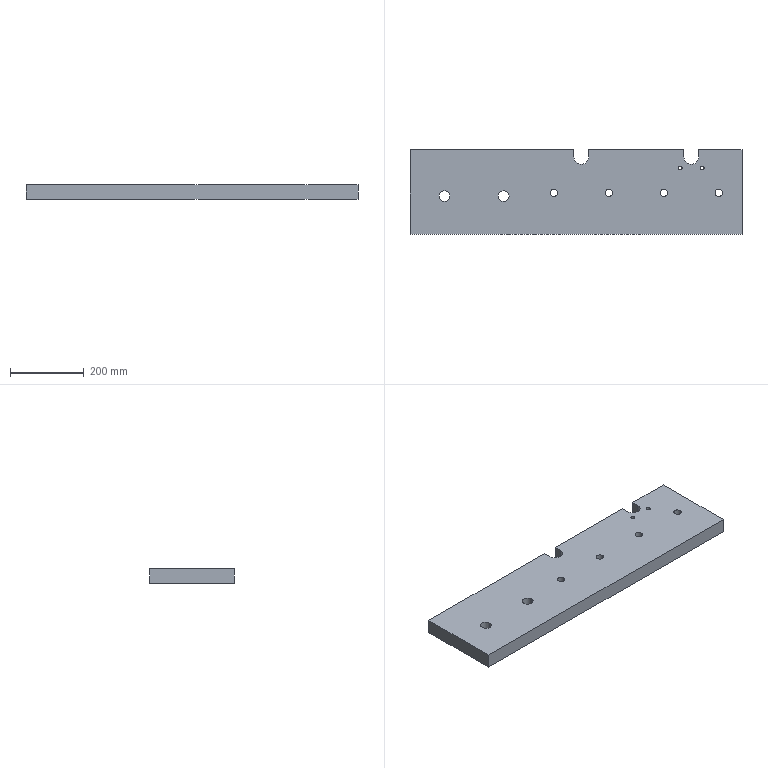Part | SolidWorks | features ICE 4, LPattern 2, Extrusion 1 | 1 solid | 30 faces | box 900 x 230 x 40 mm | volume 8056344 mm3 | cylinder 18 | plane 12 | commonest cylinder face diameters 20 x8 10 x4 29 x4 40 x2
STEP:
#1=CARTESIAN_POINT('',(-341.6,-11.,20.));
#2=VERTEX_POINT('',#1);
#3=CARTESIAN_POINT('',(-370.6,-11.,20.));
#4=VERTEX_POINT('',#3);
#5=CARTESIAN_POINT('',(-356.1,-11.,20.));
#6=DIRECTION('',(0.,0.,-1.));
#7=DIRECTION('',(-1.,0.,0.));
#8=AXIS2_PLACEMENT_3D('',#5,#6,#7);
#9=CIRCLE('',#8,14.5);
#10=EDGE_CURVE('',#2,#4,#9,.T.);
#11=ORIENTED_EDGE('',*,*,#10,.F.);
#12=CARTESIAN_POINT('',(-341.6,-11.,-20.));
#13=VERTEX_POINT('',#12);
#14=CARTESIAN_POINT('',(-341.6,-11.,20.));
#15=DIRECTION('',(0.,0.,-1.));
#16=VECTOR('',#15,1000.);
#17=LINE('',#14,#16);
#18=EDGE_CURVE('',#2,#13,#17,.T.);
#19=ORIENTED_EDGE('',*,*,#18,.T.);
#20=CARTESIAN_POINT('',(-370.6,-11.,-20.));
#21=VERTEX_POINT('',#20);
#22=CARTESIAN_POINT('',(-356.1,-11.,-20.));
#23=DIRECTION('',(0.,0.,-1.));
#24=DIRECTION('',(-1.,0.,0.));
#25=AXIS2_PLACEMENT_3D('',#22,#23,#24);
#26=CIRCLE('',#25,14.5);
#27=EDGE_CURVE('',#13,#21,#26,.T.);
#28=ORIENTED_EDGE('',*,*,#27,.T.);
#29=CARTESIAN_POINT('',(-370.6,-11.,20.));
#30=DIRECTION('',(0.,0.,-1.));
#31=VECTOR('',#30,1000.);
#32=LINE('',#29,#31);
#33=EDGE_CURVE('',#4,#21,#32,.T.);
#34=ORIENTED_EDGE('',*,*,#33,.F.);
#35=EDGE_LOOP('',(#11,#19,#28,#34));
#36=FACE_OUTER_BOUND('',#35,.T.);
#37=CARTESIAN_POINT('',(-356.1,-11.,20.));
#38=DIRECTION('',(0.,0.,-1.));
#39=DIRECTION('',(-1.,0.,0.));
#40=AXIS2_PLACEMENT_3D('',#37,#38,#39);
#41=CYLINDRICAL_SURFACE('',#40,14.5);
#42=ADVANCED_FACE('',(#36),#41,.F.);
#43=CARTESIAN_POINT('',(-181.6,-11.,20.));
#44=VERTEX_POINT('',#43);
#45=CARTESIAN_POINT('',(-210.6,-11.,20.));
#46=VERTEX_POINT('',#45);
#47=CARTESIAN_POINT('',(-196.1,-11.,20.));
#48=DIRECTION('',(0.,0.,-1.));
#49=DIRECTION('',(-1.,0.,0.));
#50=AXIS2_PLACEMENT_3D('',#47,#48,#49);
#51=CIRCLE('',#50,14.5);
#52=EDGE_CURVE('',#44,#46,#51,.T.);
#53=ORIENTED_EDGE('',*,*,#52,.F.);
#54=CARTESIAN_POINT('',(-181.6,-11.,-20.));
#55=VERTEX_POINT('',#54);
#56=CARTESIAN_POINT('',(-181.6,-11.,20.));
#57=DIRECTION('',(0.,0.,-1.));
#58=VECTOR('',#57,1000.);
#59=LINE('',#56,#58);
#60=EDGE_CURVE('',#44,#55,#59,.T.);
#61=ORIENTED_EDGE('',*,*,#60,.T.);
#62=CARTESIAN_POINT('',(-210.6,-11.,-20.));
#63=VERTEX_POINT('',#62);
#64=CARTESIAN_POINT('',(-196.1,-11.,-20.));
#65=DIRECTION('',(0.,0.,-1.));
#66=DIRECTION('',(-1.,0.,0.));
#67=AXIS2_PLACEMENT_3D('',#64,#65,#66);
#68=CIRCLE('',#67,14.5);
#69=EDGE_CURVE('',#55,#63,#68,.T.);
#70=ORIENTED_EDGE('',*,*,#69,.T.);
#71=CARTESIAN_POINT('',(-210.6,-11.,20.));
#72=DIRECTION('',(0.,0.,-1.));
#73=VECTOR('',#72,1000.);
#74=LINE('',#71,#73);
#75=EDGE_CURVE('',#46,#63,#74,.T.);
#76=ORIENTED_EDGE('',*,*,#75,.F.);
#77=EDGE_LOOP('',(#53,#61,#70,#76));
#78=FACE_OUTER_BOUND('',#77,.T.);
#79=CARTESIAN_POINT('',(-196.1,-11.,20.));
#80=DIRECTION('',(0.,0.,-1.));
#81=DIRECTION('',(-1.,0.,0.));
#82=AXIS2_PLACEMENT_3D('',#79,#80,#81);
#83=CYLINDRICAL_SURFACE('',#82,14.5);
#84=ADVANCED_FACE('',(#78),#83,.F.);
#85=CARTESIAN_POINT('',(347.5,65.,20.));
#86=VERTEX_POINT('',#85);
#87=CARTESIAN_POINT('',(337.5,65.,20.));
#88=VERTEX_POINT('',#87);
#89=CARTESIAN_POINT('',(342.5,65.,20.));
#90=DIRECTION('',(0.,0.,-1.));
#91=DIRECTION('',(-1.,0.,0.));
#92=AXIS2_PLACEMENT_3D('',#89,#90,#91);
#93=CIRCLE('',#92,5.);
#94=EDGE_CURVE('',#86,#88,#93,.T.);
#95=ORIENTED_EDGE('',*,*,#94,.F.);
#96=CARTESIAN_POINT('',(347.5,65.,-20.));
#97=VERTEX_POINT('',#96);
#98=CARTESIAN_POINT('',(347.5,65.,20.));
#99=DIRECTION('',(0.,0.,-1.));
#100=VECTOR('',#99,1000.);
#101=LINE('',#98,#100);
#102=EDGE_CURVE('',#86,#97,#101,.T.);
#103=ORIENTED_EDGE('',*,*,#102,.T.);
#104=CARTESIAN_POINT('',(337.5,65.,-20.));
#105=VERTEX_POINT('',#104);
#106=CARTESIAN_POINT('',(342.5,65.,-20.));
#107=DIRECTION('',(0.,0.,-1.));
#108=DIRECTION('',(-1.,0.,0.));
#109=AXIS2_PLACEMENT_3D('',#106,#107,#108);
#110=CIRCLE('',#109,5.);
#111=EDGE_CURVE('',#97,#105,#110,.T.);
#112=ORIENTED_EDGE('',*,*,#111,.T.);
#113=CARTESIAN_POINT('',(337.5,65.,20.));
#114=DIRECTION('',(0.,0.,-1.));
#115=VECTOR('',#114,1000.);
#116=LINE('',#113,#115);
#117=EDGE_CURVE('',#88,#105,#116,.T.);
#118=ORIENTED_EDGE('',*,*,#117,.F.);
#119=EDGE_LOOP('',(#95,#103,#112,#118));
#120=FACE_OUTER_BOUND('',#119,.T.);
#121=CARTESIAN_POINT('',(342.5,65.,20.));
#122=DIRECTION('',(0.,0.,-1.));
#123=DIRECTION('',(-1.,0.,0.));
#124=AXIS2_PLACEMENT_3D('',#121,#122,#123);
#125=CYLINDRICAL_SURFACE('',#124,5.);
#126=ADVANCED_FACE('',(#120),#125,.F.);
#127=CARTESIAN_POINT('',(287.5,65.,20.));
#128=VERTEX_POINT('',#127);
#129=CARTESIAN_POINT('',(277.5,65.,20.));
#130=VERTEX_POINT('',#129);
#131=CARTESIAN_POINT('',(282.5,65.,20.));
#132=DIRECTION('',(0.,0.,-1.));
#133=DIRECTION('',(1.,0.,0.));
#134=AXIS2_PLACEMENT_3D('',#131,#132,#133);
#135=CIRCLE('',#134,5.);
#136=EDGE_CURVE('',#128,#130,#135,.T.);
#137=ORIENTED_EDGE('',*,*,#136,.F.);
#138=CARTESIAN_POINT('',(287.5,65.,-20.));
#139=VERTEX_POINT('',#138);
#140=CARTESIAN_POINT('',(287.5,65.,20.));
#141=DIRECTION('',(0.,0.,-1.));
#142=VECTOR('',#141,1000.);
#143=LINE('',#140,#142);
#144=EDGE_CURVE('',#128,#139,#143,.T.);
#145=ORIENTED_EDGE('',*,*,#144,.T.);
#146=CARTESIAN_POINT('',(277.5,65.,-20.));
#147=VERTEX_POINT('',#146);
#148=CARTESIAN_POINT('',(282.5,65.,-20.));
#149=DIRECTION('',(0.,0.,-1.));
#150=DIRECTION('',(1.,0.,0.));
#151=AXIS2_PLACEMENT_3D('',#148,#149,#150);
#152=CIRCLE('',#151,5.);
#153=EDGE_CURVE('',#139,#147,#152,.T.);
#154=ORIENTED_EDGE('',*,*,#153,.T.);
#155=CARTESIAN_POINT('',(277.5,65.,20.));
#156=DIRECTION('',(0.,0.,-1.));
#157=VECTOR('',#156,1000.);
#158=LINE('',#155,#157);
#159=EDGE_CURVE('',#130,#147,#158,.T.);
#160=ORIENTED_EDGE('',*,*,#159,.F.);
#161=EDGE_LOOP('',(#137,#145,#154,#160));
#162=FACE_OUTER_BOUND('',#161,.T.);
#163=CARTESIAN_POINT('',(282.5,65.,20.));
#164=DIRECTION('',(0.,0.,-1.));
#165=DIRECTION('',(-1.,0.,0.));
#166=AXIS2_PLACEMENT_3D('',#163,#164,#165);
#167=CYLINDRICAL_SURFACE('',#166,5.);
#168=ADVANCED_FACE('',(#162),#167,.F.);
#169=CARTESIAN_POINT('',(228.,-2.5,-20.));
#170=VERTEX_POINT('',#169);
#171=CARTESIAN_POINT('',(248.,-2.5,-20.));
#172=VERTEX_POINT('',#171);
#173=CARTESIAN_POINT('',(238.,-2.5,-20.));
#174=DIRECTION('',(0.,0.,1.));
#175=DIRECTION('',(1.,0.,0.));
#176=AXIS2_PLACEMENT_3D('',#173,#174,#175);
#177=CIRCLE('',#176,10.);
#178=EDGE_CURVE('',#170,#172,#177,.T.);
#179=ORIENTED_EDGE('',*,*,#178,.F.);
#180=CARTESIAN_POINT('',(228.,-2.5,20.));
#181=VERTEX_POINT('',#180);
#182=CARTESIAN_POINT('',(228.,-2.5,-20.));
#183=DIRECTION('',(0.,0.,1.));
#184=VECTOR('',#183,1000.);
#185=LINE('',#182,#184);
#186=EDGE_CURVE('',#170,#181,#185,.T.);
#187=ORIENTED_EDGE('',*,*,#186,.T.);
#188=CARTESIAN_POINT('',(248.,-2.5,20.));
#189=VERTEX_POINT('',#188);
#190=CARTESIAN_POINT('',(238.,-2.5,20.));
#191=DIRECTION('',(0.,0.,1.));
#192=DIRECTION('',(1.,0.,0.));
#193=AXIS2_PLACEMENT_3D('',#190,#191,#192);
#194=CIRCLE('',#193,10.);
#195=EDGE_CURVE('',#181,#189,#194,.T.);
#196=ORIENTED_EDGE('',*,*,#195,.T.);
#197=CARTESIAN_POINT('',(248.,-2.5,-20.));
#198=DIRECTION('',(0.,0.,1.));
#199=VECTOR('',#198,1000.);
#200=LINE('',#197,#199);
#201=EDGE_CURVE('',#172,#189,#200,.T.);
#202=ORIENTED_EDGE('',*,*,#201,.F.);
#203=EDGE_LOOP('',(#179,#187,#196,#202));
#204=FACE_OUTER_BOUND('',#203,.T.);
#205=CARTESIAN_POINT('',(238.,-2.5,-20.));
#206=DIRECTION('',(0.,0.,1.));
#207=DIRECTION('',(1.,0.,0.));
#208=AXIS2_PLACEMENT_3D('',#205,#206,#207);
#209=CYLINDRICAL_SURFACE('',#208,10.);
#210=ADVANCED_FACE('',(#204),#209,.F.);
#211=CARTESIAN_POINT('',(377.,-2.5,-20.));
#212=VERTEX_POINT('',#211);
#213=CARTESIAN_POINT('',(397.,-2.5,-20.));
#214=VERTEX_POINT('',#213);
#215=CARTESIAN_POINT('',(387.,-2.5,-20.));
#216=DIRECTION('',(0.,0.,1.));
#217=DIRECTION('',(1.,0.,0.));
#218=AXIS2_PLACEMENT_3D('',#215,#216,#217);
#219=CIRCLE('',#218,10.);
#220=EDGE_CURVE('',#212,#214,#219,.T.);
#221=ORIENTED_EDGE('',*,*,#220,.F.);
#222=CARTESIAN_POINT('',(377.,-2.5,20.));
#223=VERTEX_POINT('',#222);
#224=CARTESIAN_POINT('',(377.,-2.5,-20.));
#225=DIRECTION('',(0.,0.,1.));
#226=VECTOR('',#225,1000.);
#227=LINE('',#224,#226);
#228=EDGE_CURVE('',#212,#223,#227,.T.);
#229=ORIENTED_EDGE('',*,*,#228,.T.);
#230=CARTESIAN_POINT('',(397.,-2.5,20.));
#231=VERTEX_POINT('',#230);
#232=CARTESIAN_POINT('',(387.,-2.5,20.));
#233=DIRECTION('',(0.,0.,1.));
#234=DIRECTION('',(1.,0.,0.));
#235=AXIS2_PLACEMENT_3D('',#232,#233,#234);
#236=CIRCLE('',#235,10.);
#237=EDGE_CURVE('',#223,#231,#236,.T.);
#238=ORIENTED_EDGE('',*,*,#237,.T.);
#239=CARTESIAN_POINT('',(397.,-2.5,-20.));
#240=DIRECTION('',(0.,0.,1.));
#241=VECTOR('',#240,1000.);
#242=LINE('',#239,#241);
#243=EDGE_CURVE('',#214,#231,#242,.T.);
#244=ORIENTED_EDGE('',*,*,#243,.F.);
#245=EDGE_LOOP('',(#221,#229,#238,#244));
#246=FACE_OUTER_BOUND('',#245,.T.);
#247=CARTESIAN_POINT('',(387.,-2.5,-20.));
#248=DIRECTION('',(0.,0.,1.));
#249=DIRECTION('',(1.,0.,0.));
#250=AXIS2_PLACEMENT_3D('',#247,#248,#249);
#251=CYLINDRICAL_SURFACE('',#250,10.);
#252=ADVANCED_FACE('',(#246),#251,.F.);
#253=CARTESIAN_POINT('',(79.,-2.5,-20.));
#254=VERTEX_POINT('',#253);
#255=CARTESIAN_POINT('',(99.,-2.5,-20.));
#256=VERTEX_POINT('',#255);
#257=CARTESIAN_POINT('',(89.,-2.5,-20.));
#258=DIRECTION('',(0.,0.,1.));
#259=DIRECTION('',(1.,0.,0.));
#260=AXIS2_PLACEMENT_3D('',#257,#258,#259);
#261=CIRCLE('',#260,10.);
#262=EDGE_CURVE('',#254,#256,#261,.T.);
#263=ORIENTED_EDGE('',*,*,#262,.F.);
#264=CARTESIAN_POINT('',(79.,-2.5,20.));
#265=VERTEX_POINT('',#264);
#266=CARTESIAN_POINT('',(79.,-2.5,-20.));
#267=DIRECTION('',(0.,0.,1.));
#268=VECTOR('',#267,1000.);
#269=LINE('',#266,#268);
#270=EDGE_CURVE('',#254,#265,#269,.T.);
#271=ORIENTED_EDGE('',*,*,#270,.T.);
#272=CARTESIAN_POINT('',(99.,-2.5,20.));
#273=VERTEX_POINT('',#272);
#274=CARTESIAN_POINT('',(89.,-2.5,20.));
#275=DIRECTION('',(0.,0.,1.));
#276=DIRECTION('',(1.,0.,0.));
#277=AXIS2_PLACEMENT_3D('',#274,#275,#276);
#278=CIRCLE('',#277,10.);
#279=EDGE_CURVE('',#265,#273,#278,.T.);
#280=ORIENTED_EDGE('',*,*,#279,.T.);
#281=CARTESIAN_POINT('',(99.,-2.5,-20.));
#282=DIRECTION('',(0.,0.,1.));
#283=VECTOR('',#282,1000.);
#284=LINE('',#281,#283);
#285=EDGE_CURVE('',#256,#273,#284,.T.);
#286=ORIENTED_EDGE('',*,*,#285,.F.);
#287=EDGE_LOOP('',(#263,#271,#280,#286));
#288=FACE_OUTER_BOUND('',#287,.T.);
#289=CARTESIAN_POINT('',(89.,-2.5,-20.));
#290=DIRECTION('',(0.,0.,1.));
#291=DIRECTION('',(1.,0.,0.));
#292=AXIS2_PLACEMENT_3D('',#289,#290,#291);
#293=CYLINDRICAL_SURFACE('',#292,10.);
#294=ADVANCED_FACE('',(#288),#293,.F.);
#295=CARTESIAN_POINT('',(-70.,-2.5,-20.));
#296=VERTEX_POINT('',#295);
#297=CARTESIAN_POINT('',(-50.,-2.5,-20.));
#298=VERTEX_POINT('',#297);
#299=CARTESIAN_POINT('',(-60.,-2.5,-20.));
#300=DIRECTION('',(0.,0.,1.));
#301=DIRECTION('',(1.,0.,0.));
#302=AXIS2_PLACEMENT_3D('',#299,#300,#301);
#303=CIRCLE('',#302,10.);
#304=EDGE_CURVE('',#296,#298,#303,.T.);
#305=ORIENTED_EDGE('',*,*,#304,.F.);
#306=CARTESIAN_POINT('',(-70.,-2.5,20.));
#307=VERTEX_POINT('',#306);
#308=CARTESIAN_POINT('',(-70.,-2.5,-20.));
#309=DIRECTION('',(0.,0.,1.));
#310=VECTOR('',#309,1000.);
#311=LINE('',#308,#310);
#312=EDGE_CURVE('',#296,#307,#311,.T.);
#313=ORIENTED_EDGE('',*,*,#312,.T.);
#314=CARTESIAN_POINT('',(-50.,-2.5,20.));
#315=VERTEX_POINT('',#314);
#316=CARTESIAN_POINT('',(-60.,-2.5,20.));
#317=DIRECTION('',(0.,0.,1.));
#318=DIRECTION('',(1.,0.,0.));
#319=AXIS2_PLACEMENT_3D('',#316,#317,#318);
#320=CIRCLE('',#319,10.);
#321=EDGE_CURVE('',#307,#315,#320,.T.);
#322=ORIENTED_EDGE('',*,*,#321,.T.);
#323=CARTESIAN_POINT('',(-50.,-2.5,-20.));
#324=DIRECTION('',(0.,0.,1.));
#325=VECTOR('',#324,1000.);
#326=LINE('',#323,#325);
#327=EDGE_CURVE('',#298,#315,#326,.T.);
#328=ORIENTED_EDGE('',*,*,#327,.F.);
#329=EDGE_LOOP('',(#305,#313,#322,#328));
#330=FACE_OUTER_BOUND('',#329,.T.);
#331=CARTESIAN_POINT('',(-60.,-2.5,-20.));
#332=DIRECTION('',(0.,0.,1.));
#333=DIRECTION('',(1.,0.,0.));
#334=AXIS2_PLACEMENT_3D('',#331,#332,#333);
#335=CYLINDRICAL_SURFACE('',#334,10.);
#336=ADVANCED_FACE('',(#330),#335,.F.);
#337=ORIENTED_EDGE('',*,*,#312,.F.);
#338=CARTESIAN_POINT('',(-60.,-2.5,-20.));
#339=DIRECTION('',(0.,0.,1.));
#340=DIRECTION('',(1.,0.,0.));
#341=AXIS2_PLACEMENT_3D('',#338,#339,#340);
#342=CIRCLE('',#341,10.);
#343=EDGE_CURVE('',#298,#296,#342,.T.);
#344=ORIENTED_EDGE('',*,*,#343,.F.);
#345=ORIENTED_EDGE('',*,*,#327,.T.);
#346=CARTESIAN_POINT('',(-60.,-2.5,20.));
#347=DIRECTION('',(0.,0.,1.));
#348=DIRECTION('',(1.,0.,0.));
#349=AXIS2_PLACEMENT_3D('',#346,#347,#348);
#350=CIRCLE('',#349,10.);
#351=EDGE_CURVE('',#315,#307,#350,.T.);
#352=ORIENTED_EDGE('',*,*,#351,.T.);
#353=EDGE_LOOP('',(#337,#344,#345,#352));
#354=FACE_OUTER_BOUND('',#353,.T.);
#355=CARTESIAN_POINT('',(-60.,-2.5,-20.));
#356=DIRECTION('',(0.,0.,1.));
#357=DIRECTION('',(1.,0.,0.));
#358=AXIS2_PLACEMENT_3D('',#355,#356,#357);
#359=CYLINDRICAL_SURFACE('',#358,10.);
#360=ADVANCED_FACE('',(#354),#359,.F.);
#361=ORIENTED_EDGE('',*,*,#270,.F.);
#362=CARTESIAN_POINT('',(89.,-2.5,-20.));
#363=DIRECTION('',(0.,0.,1.));
#364=DIRECTION('',(1.,0.,0.));
#365=AXIS2_PLACEMENT_3D('',#362,#363,#364);
#366=CIRCLE('',#365,10.);
#367=EDGE_CURVE('',#256,#254,#366,.T.);
#368=ORIENTED_EDGE('',*,*,#367,.F.);
#369=ORIENTED_EDGE('',*,*,#285,.T.);
#370=CARTESIAN_POINT('',(89.,-2.5,20.));
#371=DIRECTION('',(0.,0.,1.));
#372=DIRECTION('',(1.,0.,0.));
#373=AXIS2_PLACEMENT_3D('',#370,#371,#372);
#374=CIRCLE('',#373,10.);
#375=EDGE_CURVE('',#273,#265,#374,.T.);
#376=ORIENTED_EDGE('',*,*,#375,.T.);
#377=EDGE_LOOP('',(#361,#368,#369,#376));
#378=FACE_OUTER_BOUND('',#377,.T.);
#379=CARTESIAN_POINT('',(89.,-2.5,-20.));
#380=DIRECTION('',(0.,0.,1.));
#381=DIRECTION('',(1.,0.,0.));
#382=AXIS2_PLACEMENT_3D('',#379,#380,#381);
#383=CYLINDRICAL_SURFACE('',#382,10.);
#384=ADVANCED_FACE('',(#378),#383,.F.);
#385=CARTESIAN_POINT('',(292.5,115.,-20.));
#386=VERTEX_POINT('',#385);
#387=CARTESIAN_POINT('',(34.5,115.,-20.));
#388=VERTEX_POINT('',#387);
#389=CARTESIAN_POINT('',(450.,115.,-20.));
#390=DIRECTION('',(-1.,0.,0.));
#391=VECTOR('',#390,1000.);
#392=LINE('',#389,#391);
#393=EDGE_CURVE('',#386,#388,#392,.T.);
#394=ORIENTED_EDGE('',*,*,#393,.T.);
#395=CARTESIAN_POINT('',(34.5,115.,20.));
#396=VERTEX_POINT('',#395);
#397=CARTESIAN_POINT('',(34.5,115.,-20.));
#398=DIRECTION('',(0.,0.,1.));
#399=VECTOR('',#398,1000.);
#400=LINE('',#397,#399);
#401=EDGE_CURVE('',#388,#396,#400,.T.);
#402=ORIENTED_EDGE('',*,*,#401,.T.);
#403=CARTESIAN_POINT('',(292.5,115.,20.));
#404=VERTEX_POINT('',#403);
#405=CARTESIAN_POINT('',(450.,115.,20.));
#406=DIRECTION('',(-1.,0.,0.));
#407=VECTOR('',#406,1000.);
#408=LINE('',#405,#407);
#409=EDGE_CURVE('',#404,#396,#408,.T.);
#410=ORIENTED_EDGE('',*,*,#409,.F.);
#411=CARTESIAN_POINT('',(292.5,115.,-20.));
#412=DIRECTION('',(0.,0.,1.));
#413=VECTOR('',#412,1000.);
#414=LINE('',#411,#413);
#415=EDGE_CURVE('',#386,#404,#414,.T.);
#416=ORIENTED_EDGE('',*,*,#415,.F.);
#417=EDGE_LOOP('',(#394,#402,#410,#416));
#418=FACE_OUTER_BOUND('',#417,.T.);
#419=CARTESIAN_POINT('',(450.,115.,20.));
#420=DIRECTION('',(0.,-1.,0.));
#421=DIRECTION('',(1.,0.,0.));
#422=AXIS2_PLACEMENT_3D('',#419,#420,#421);
#423=PLANE('',#422);
#424=ADVANCED_FACE('',(#418),#423,.F.);
#425=CARTESIAN_POINT('',(450.,115.,-20.));
#426=VERTEX_POINT('',#425);
#427=CARTESIAN_POINT('',(332.5,115.,-20.));
#428=VERTEX_POINT('',#427);
#429=CARTESIAN_POINT('',(450.,115.,-20.));
#430=DIRECTION('',(-1.,0.,0.));
#431=VECTOR('',#430,1000.);
#432=LINE('',#429,#431);
#433=EDGE_CURVE('',#426,#428,#432,.T.);
#434=ORIENTED_EDGE('',*,*,#433,.T.);
#435=CARTESIAN_POINT('',(332.5,115.,20.));
#436=VERTEX_POINT('',#435);
#437=CARTESIAN_POINT('',(332.5,115.,-20.));
#438=DIRECTION('',(0.,0.,1.));
#439=VECTOR('',#438,1000.);
#440=LINE('',#437,#439);
#441=EDGE_CURVE('',#428,#436,#440,.T.);
#442=ORIENTED_EDGE('',*,*,#441,.T.);
#443=CARTESIAN_POINT('',(450.,115.,20.));
#444=VERTEX_POINT('',#443);
#445=CARTESIAN_POINT('',(450.,115.,20.));
#446=DIRECTION('',(-1.,0.,0.));
#447=VECTOR('',#446,1000.);
#448=LINE('',#445,#447);
#449=EDGE_CURVE('',#444,#436,#448,.T.);
#450=ORIENTED_EDGE('',*,*,#449,.F.);
#451=CARTESIAN_POINT('',(450.,115.,20.));
#452=DIRECTION('',(0.,0.,-1.));
#453=VECTOR('',#452,1000.);
#454=LINE('',#451,#453);
#455=EDGE_CURVE('',#444,#426,#454,.T.);
#456=ORIENTED_EDGE('',*,*,#455,.T.);
#457=EDGE_LOOP('',(#434,#442,#450,#456));
#458=FACE_OUTER_BOUND('',#457,.T.);
#459=CARTESIAN_POINT('',(450.,115.,20.));
#460=DIRECTION('',(0.,-1.,0.));
#461=DIRECTION('',(1.,0.,0.));
#462=AXIS2_PLACEMENT_3D('',#459,#460,#461);
#463=PLANE('',#462);
#464=ADVANCED_FACE('',(#458),#463,.F.);
#465=CARTESIAN_POINT('',(-450.,115.,-20.));
#466=VERTEX_POINT('',#465);
#467=CARTESIAN_POINT('',(-450.,-115.,-20.));
#468=VERTEX_POINT('',#467);
#469=CARTESIAN_POINT('',(-450.,-115.,-20.));
#470=DIRECTION('',(0.,-1.,0.));
#471=VECTOR('',#470,1000.);
#472=LINE('',#469,#471);
#473=EDGE_CURVE('',#466,#468,#472,.T.);
#474=ORIENTED_EDGE('',*,*,#473,.T.);
#475=CARTESIAN_POINT('',(-450.,-115.,20.));
#476=VERTEX_POINT('',#475);
#477=CARTESIAN_POINT('',(-450.,-115.,20.));
#478=DIRECTION('',(0.,0.,-1.));
#479=VECTOR('',#478,1000.);
#480=LINE('',#477,#479);
#481=EDGE_CURVE('',#476,#468,#480,.T.);
#482=ORIENTED_EDGE('',*,*,#481,.F.);
#483=CARTESIAN_POINT('',(-450.,115.,20.));
#484=VERTEX_POINT('',#483);
#485=CARTESIAN_POINT('',(-450.,-115.,20.));
#486=DIRECTION('',(0.,-1.,0.));
#487=VECTOR('',#486,1000.);
#488=LINE('',#485,#487);
#489=EDGE_CURVE('',#484,#476,#488,.T.);
#490=ORIENTED_EDGE('',*,*,#489,.F.);
#491=CARTESIAN_POINT('',(-450.,115.,20.));
#492=DIRECTION('',(0.,0.,-1.));
#493=VECTOR('',#492,1000.);
#494=LINE('',#491,#493);
#495=EDGE_CURVE('',#484,#466,#494,.T.);
#496=ORIENTED_EDGE('',*,*,#495,.T.);
#497=EDGE_LOOP('',(#474,#482,#490,#496));
#498=FACE_OUTER_BOUND('',#497,.T.);
#499=CARTESIAN_POINT('',(-450.,-115.,20.));
#500=DIRECTION('',(1.,0.,0.));
#501=DIRECTION('',(0.,0.,-1.));
#502=AXIS2_PLACEMENT_3D('',#499,#500,#501);
#503=PLANE('',#502);
#504=ADVANCED_FACE('',(#498),#503,.F.);
#505=CARTESIAN_POINT('',(450.,-115.,-20.));
#506=VERTEX_POINT('',#505);
#507=CARTESIAN_POINT('',(450.,-115.,-20.));
#508=DIRECTION('',(1.,0.,0.));
#509=VECTOR('',#508,1000.);
#510=LINE('',#507,#509);
#511=EDGE_CURVE('',#468,#506,#510,.T.);
#512=ORIENTED_EDGE('',*,*,#511,.T.);
#513=CARTESIAN_POINT('',(450.,-115.,20.));
#514=VERTEX_POINT('',#513);
#515=CARTESIAN_POINT('',(450.,-115.,20.));
#516=DIRECTION('',(0.,0.,-1.));
#517=VECTOR('',#516,1000.);
#518=LINE('',#515,#517);
#519=EDGE_CURVE('',#514,#506,#518,.T.);
#520=ORIENTED_EDGE('',*,*,#519,.F.);
#521=CARTESIAN_POINT('',(450.,-115.,20.));
#522=DIRECTION('',(1.,0.,0.));
#523=VECTOR('',#522,1000.);
#524=LINE('',#521,#523);
#525=EDGE_CURVE('',#476,#514,#524,.T.);
#526=ORIENTED_EDGE('',*,*,#525,.F.);
#527=ORIENTED_EDGE('',*,*,#481,.T.);
#528=EDGE_LOOP('',(#512,#520,#526,#527));
#529=FACE_OUTER_BOUND('',#528,.T.);
#530=CARTESIAN_POINT('',(450.,-115.,20.));
#531=DIRECTION('',(0.,1.,0.));
#532=DIRECTION('',(-1.,0.,0.));
#533=AXIS2_PLACEMENT_3D('',#530,#531,#532);
#534=PLANE('',#533);
#535=ADVANCED_FACE('',(#529),#534,.F.);
#536=CARTESIAN_POINT('',(450.,-115.,-20.));
#537=DIRECTION('',(0.,1.,0.));
#538=VECTOR('',#537,1000.);
#539=LINE('',#536,#538);
#540=EDGE_CURVE('',#506,#426,#539,.T.);
#541=ORIENTED_EDGE('',*,*,#540,.T.);
#542=ORIENTED_EDGE('',*,*,#455,.F.);
#543=CARTESIAN_POINT('',(450.,-115.,20.));
#544=DIRECTION('',(0.,1.,0.));
#545=VECTOR('',#544,1000.);
#546=LINE('',#543,#545);
#547=EDGE_CURVE('',#514,#444,#546,.T.);
#548=ORIENTED_EDGE('',*,*,#547,.F.);
#549=ORIENTED_EDGE('',*,*,#519,.T.);
#550=EDGE_LOOP('',(#541,#542,#548,#549));
#551=FACE_OUTER_BOUND('',#550,.T.);
#552=CARTESIAN_POINT('',(450.,-115.,20.));
#553=DIRECTION('',(-1.,0.,0.));
#554=DIRECTION('',(0.,0.,1.));
#555=AXIS2_PLACEMENT_3D('',#552,#553,#554);
#556=PLANE('',#555);
#557=ADVANCED_FACE('',(#551),#556,.F.);
#558=CARTESIAN_POINT('',(-5.5,115.,20.));
#559=VERTEX_POINT('',#558);
#560=CARTESIAN_POINT('',(450.,115.,20.));
#561=DIRECTION('',(-1.,0.,0.));
#562=VECTOR('',#561,1000.);
#563=LINE('',#560,#562);
#564=EDGE_CURVE('',#559,#484,#563,.T.);
#565=ORIENTED_EDGE('',*,*,#564,.F.);
#566=CARTESIAN_POINT('',(-5.5,115.,-20.));
#567=VERTEX_POINT('',#566);
#568=CARTESIAN_POINT('',(-5.5,115.,-20.));
#569=DIRECTION('',(0.,0.,1.));
#570=VECTOR('',#569,1000.);
#571=LINE('',#568,#570);
#572=EDGE_CURVE('',#567,#559,#571,.T.);
#573=ORIENTED_EDGE('',*,*,#572,.F.);
#574=CARTESIAN_POINT('',(450.,115.,-20.));
#575=DIRECTION('',(-1.,0.,0.));
#576=VECTOR('',#575,1000.);
#577=LINE('',#574,#576);
#578=EDGE_CURVE('',#567,#466,#577,.T.);
#579=ORIENTED_EDGE('',*,*,#578,.T.);
#580=ORIENTED_EDGE('',*,*,#495,.F.);
#581=EDGE_LOOP('',(#565,#573,#579,#580));
#582=FACE_OUTER_BOUND('',#581,.T.);
#583=CARTESIAN_POINT('',(450.,115.,20.));
#584=DIRECTION('',(0.,-1.,0.));
#585=DIRECTION('',(1.,0.,0.));
#586=AXIS2_PLACEMENT_3D('',#583,#584,#585);
#587=PLANE('',#586);
#588=ADVANCED_FACE('',(#582),#587,.F.);
#589=CARTESIAN_POINT('',(-356.1,-11.,20.));
#590=DIRECTION('',(0.,0.,-1.));
#591=DIRECTION('',(-1.,0.,0.));
#592=AXIS2_PLACEMENT_3D('',#589,#590,#591);
#593=CIRCLE('',#592,14.5);
#594=EDGE_CURVE('',#4,#2,#593,.T.);
#595=ORIENTED_EDGE('',*,*,#594,.T.);
#596=ORIENTED_EDGE('',*,*,#10,.T.);
#597=EDGE_LOOP('',(#595,#596));
#598=FACE_BOUND('',#597,.T.);
#599=CARTESIAN_POINT('',(-196.1,-11.,20.));
#600=DIRECTION('',(0.,0.,-1.));
#601=DIRECTION('',(-1.,0.,0.));
#602=AXIS2_PLACEMENT_3D('',#599,#600,#601);
#603=CIRCLE('',#602,14.5);
#604=EDGE_CURVE('',#46,#44,#603,.T.);
#605=ORIENTED_EDGE('',*,*,#604,.T.);
#606=ORIENTED_EDGE('',*,*,#52,.T.);
#607=EDGE_LOOP('',(#605,#606));
#608=FACE_BOUND('',#607,.T.);
#609=CARTESIAN_POINT('',(342.5,65.,20.));
#610=DIRECTION('',(0.,0.,-1.));
#611=DIRECTION('',(-1.,0.,0.));
#612=AXIS2_PLACEMENT_3D('',#609,#610,#611);
#613=CIRCLE('',#612,5.);
#614=EDGE_CURVE('',#88,#86,#613,.T.);
#615=ORIENTED_EDGE('',*,*,#614,.T.);
#616=ORIENTED_EDGE('',*,*,#94,.T.);
#617=EDGE_LOOP('',(#615,#616));
#618=FACE_BOUND('',#617,.T.);
#619=CARTESIAN_POINT('',(282.5,65.,20.));
#620=DIRECTION('',(0.,0.,-1.));
#621=DIRECTION('',(1.,0.,0.));
#622=AXIS2_PLACEMENT_3D('',#619,#620,#621);
#623=CIRCLE('',#622,5.);
#624=EDGE_CURVE('',#130,#128,#623,.T.);
#625=ORIENTED_EDGE('',*,*,#624,.T.);
#626=ORIENTED_EDGE('',*,*,#136,.T.);
#627=EDGE_LOOP('',(#625,#626));
#628=FACE_BOUND('',#627,.T.);
#629=CARTESIAN_POINT('',(238.,-2.5,20.));
#630=DIRECTION('',(0.,0.,1.));
#631=DIRECTION('',(1.,0.,0.));
#632=AXIS2_PLACEMENT_3D('',#629,#630,#631);
#633=CIRCLE('',#632,10.);
#634=EDGE_CURVE('',#189,#181,#633,.T.);
#635=ORIENTED_EDGE('',*,*,#634,.F.);
#636=ORIENTED_EDGE('',*,*,#195,.F.);
#637=EDGE_LOOP('',(#635,#636));
#638=FACE_BOUND('',#637,.T.);
#639=CARTESIAN_POINT('',(34.5,95.,20.));
#640=VERTEX_POINT('',#639);
#641=CARTESIAN_POINT('',(34.5,115.,20.));
#642=DIRECTION('',(0.,1.,0.));
#643=VECTOR('',#642,1000.);
#644=LINE('',#641,#643);
#645=EDGE_CURVE('',#640,#396,#644,.T.);
#646=ORIENTED_EDGE('',*,*,#645,.F.);
#647=CARTESIAN_POINT('',(-5.5,95.,20.));
#648=VERTEX_POINT('',#647);
#649=CARTESIAN_POINT('',(14.5,95.,20.));
#650=DIRECTION('',(0.,0.,1.));
#651=DIRECTION('',(1.,0.,0.));
#652=AXIS2_PLACEMENT_3D('',#649,#650,#651);
#653=CIRCLE('',#652,20.);
#654=EDGE_CURVE('',#648,#640,#653,.T.);
#655=ORIENTED_EDGE('',*,*,#654,.F.);
#656=CARTESIAN_POINT('',(-5.5,115.,20.));
#657=DIRECTION('',(0.,-1.,0.));
#658=VECTOR('',#657,1000.);
#659=LINE('',#656,#658);
#660=EDGE_CURVE('',#559,#648,#659,.T.);
#661=ORIENTED_EDGE('',*,*,#660,.F.);
#662=ORIENTED_EDGE('',*,*,#564,.T.);
#663=ORIENTED_EDGE('',*,*,#489,.T.);
#664=ORIENTED_EDGE('',*,*,#525,.T.);
#665=ORIENTED_EDGE('',*,*,#547,.T.);
#666=ORIENTED_EDGE('',*,*,#449,.T.);
#667=CARTESIAN_POINT('',(332.5,95.,20.));
#668=VERTEX_POINT('',#667);
#669=CARTESIAN_POINT('',(332.5,115.,20.));
#670=DIRECTION('',(0.,1.,0.));
#671=VECTOR('',#670,1000.);
#672=LINE('',#669,#671);
#673=EDGE_CURVE('',#668,#436,#672,.T.);
#674=ORIENTED_EDGE('',*,*,#673,.F.);
#675=CARTESIAN_POINT('',(292.5,95.,20.));
#676=VERTEX_POINT('',#675);
#677=CARTESIAN_POINT('',(312.5,95.,20.));
#678=DIRECTION('',(0.,0.,1.));
#679=DIRECTION('',(1.,0.,0.));
#680=AXIS2_PLACEMENT_3D('',#677,#678,#679);
#681=CIRCLE('',#680,20.);
#682=EDGE_CURVE('',#676,#668,#681,.T.);
#683=ORIENTED_EDGE('',*,*,#682,.F.);
#684=CARTESIAN_POINT('',(292.5,115.,20.));
#685=DIRECTION('',(0.,-1.,0.));
#686=VECTOR('',#685,1000.);
#687=LINE('',#684,#686);
#688=EDGE_CURVE('',#404,#676,#687,.T.);
#689=ORIENTED_EDGE('',*,*,#688,.F.);
#690=ORIENTED_EDGE('',*,*,#409,.T.);
#691=EDGE_LOOP('',(#646,#655,#661,#662,#663,#664,#665,#666,#674,#683,#689,#690));
#692=FACE_OUTER_BOUND('',#691,.T.);
#693=CARTESIAN_POINT('',(387.,-2.5,20.));
#694=DIRECTION('',(0.,0.,1.));
#695=DIRECTION('',(1.,0.,0.));
#696=AXIS2_PLACEMENT_3D('',#693,#694,#695);
#697=CIRCLE('',#696,10.);
#698=EDGE_CURVE('',#231,#223,#697,.T.);
#699=ORIENTED_EDGE('',*,*,#698,.F.);
#700=ORIENTED_EDGE('',*,*,#237,.F.);
#701=EDGE_LOOP('',(#699,#700));
#702=FACE_BOUND('',#701,.T.);
#703=ORIENTED_EDGE('',*,*,#375,.F.);
#704=ORIENTED_EDGE('',*,*,#279,.F.);
#705=EDGE_LOOP('',(#703,#704));
#706=FACE_BOUND('',#705,.T.);
#707=ORIENTED_EDGE('',*,*,#351,.F.);
#708=ORIENTED_EDGE('',*,*,#321,.F.);
#709=EDGE_LOOP('',(#707,#708));
#710=FACE_BOUND('',#709,.T.);
#711=CARTESIAN_POINT('',(0.,0.,20.));
#712=DIRECTION('',(0.,0.,1.));
#713=DIRECTION('',(1.,0.,0.));
#714=AXIS2_PLACEMENT_3D('',#711,#712,#713);
#715=PLANE('',#714);
#716=ADVANCED_FACE('',(#598,#608,#618,#628,#638,#692,#702,#706,#710),#715,.T.);
#717=CARTESIAN_POINT('',(-356.1,-11.,-20.));
#718=DIRECTION('',(0.,0.,-1.));
#719=DIRECTION('',(-1.,0.,0.));
#720=AXIS2_PLACEMENT_3D('',#717,#718,#719);
#721=CIRCLE('',#720,14.5);
#722=EDGE_CURVE('',#21,#13,#721,.T.);
#723=ORIENTED_EDGE('',*,*,#722,.F.);
#724=ORIENTED_EDGE('',*,*,#27,.F.);
#725=EDGE_LOOP('',(#723,#724));
#726=FACE_BOUND('',#725,.T.);
#727=CARTESIAN_POINT('',(-196.1,-11.,-20.));
#728=DIRECTION('',(0.,0.,-1.));
#729=DIRECTION('',(-1.,0.,0.));
#730=AXIS2_PLACEMENT_3D('',#727,#728,#729);
#731=CIRCLE('',#730,14.5);
#732=EDGE_CURVE('',#63,#55,#731,.T.);
#733=ORIENTED_EDGE('',*,*,#732,.F.);
#734=ORIENTED_EDGE('',*,*,#69,.F.);
#735=EDGE_LOOP('',(#733,#734));
#736=FACE_BOUND('',#735,.T.);
#737=CARTESIAN_POINT('',(342.5,65.,-20.));
#738=DIRECTION('',(0.,0.,-1.));
#739=DIRECTION('',(-1.,0.,0.));
#740=AXIS2_PLACEMENT_3D('',#737,#738,#739);
#741=CIRCLE('',#740,5.);
#742=EDGE_CURVE('',#105,#97,#741,.T.);
#743=ORIENTED_EDGE('',*,*,#742,.F.);
#744=ORIENTED_EDGE('',*,*,#111,.F.);
#745=EDGE_LOOP('',(#743,#744));
#746=FACE_BOUND('',#745,.T.);
#747=CARTESIAN_POINT('',(282.5,65.,-20.));
#748=DIRECTION('',(0.,0.,-1.));
#749=DIRECTION('',(1.,0.,0.));
#750=AXIS2_PLACEMENT_3D('',#747,#748,#749);
#751=CIRCLE('',#750,5.);
#752=EDGE_CURVE('',#147,#139,#751,.T.);
#753=ORIENTED_EDGE('',*,*,#752,.F.);
#754=ORIENTED_EDGE('',*,*,#153,.F.);
#755=EDGE_LOOP('',(#753,#754));
#756=FACE_BOUND('',#755,.T.);
#757=CARTESIAN_POINT('',(238.,-2.5,-20.));
#758=DIRECTION('',(0.,0.,1.));
#759=DIRECTION('',(1.,0.,0.));
#760=AXIS2_PLACEMENT_3D('',#757,#758,#759);
#761=CIRCLE('',#760,10.);
#762=EDGE_CURVE('',#172,#170,#761,.T.);
#763=ORIENTED_EDGE('',*,*,#762,.T.);
#764=ORIENTED_EDGE('',*,*,#178,.T.);
#765=EDGE_LOOP('',(#763,#764));
#766=FACE_BOUND('',#765,.T.);
#767=CARTESIAN_POINT('',(387.,-2.5,-20.));
#768=DIRECTION('',(0.,0.,1.));
#769=DIRECTION('',(1.,0.,0.));
#770=AXIS2_PLACEMENT_3D('',#767,#768,#769);
#771=CIRCLE('',#770,10.);
#772=EDGE_CURVE('',#214,#212,#771,.T.);
#773=ORIENTED_EDGE('',*,*,#772,.T.);
#774=ORIENTED_EDGE('',*,*,#220,.T.);
#775=EDGE_LOOP('',(#773,#774));
#776=FACE_BOUND('',#775,.T.);
#777=CARTESIAN_POINT('',(-5.5,95.,-20.));
#778=VERTEX_POINT('',#777);
#779=CARTESIAN_POINT('',(34.5,95.,-20.));
#780=VERTEX_POINT('',#779);
#781=CARTESIAN_POINT('',(14.5,95.,-20.));
#782=DIRECTION('',(0.,0.,1.));
#783=DIRECTION('',(1.,0.,0.));
#784=AXIS2_PLACEMENT_3D('',#781,#782,#783);
#785=CIRCLE('',#784,20.);
#786=EDGE_CURVE('',#778,#780,#785,.T.);
#787=ORIENTED_EDGE('',*,*,#786,.T.);
#788=CARTESIAN_POINT('',(34.5,115.,-20.));
#789=DIRECTION('',(0.,1.,0.));
#790=VECTOR('',#789,1000.);
#791=LINE('',#788,#790);
#792=EDGE_CURVE('',#780,#388,#791,.T.);
#793=ORIENTED_EDGE('',*,*,#792,.T.);
#794=ORIENTED_EDGE('',*,*,#393,.F.);
#795=CARTESIAN_POINT('',(292.5,95.,-20.));
#796=VERTEX_POINT('',#795);
#797=CARTESIAN_POINT('',(292.5,115.,-20.));
#798=DIRECTION('',(0.,-1.,0.));
#799=VECTOR('',#798,1000.);
#800=LINE('',#797,#799);
#801=EDGE_CURVE('',#386,#796,#800,.T.);
#802=ORIENTED_EDGE('',*,*,#801,.T.);
#803=CARTESIAN_POINT('',(332.5,95.,-20.));
#804=VERTEX_POINT('',#803);
#805=CARTESIAN_POINT('',(312.5,95.,-20.));
#806=DIRECTION('',(0.,0.,1.));
#807=DIRECTION('',(1.,0.,0.));
#808=AXIS2_PLACEMENT_3D('',#805,#806,#807);
#809=CIRCLE('',#808,20.);
#810=EDGE_CURVE('',#796,#804,#809,.T.);
#811=ORIENTED_EDGE('',*,*,#810,.T.);
#812=CARTESIAN_POINT('',(332.5,115.,-20.));
#813=DIRECTION('',(0.,1.,0.));
#814=VECTOR('',#813,1000.);
#815=LINE('',#812,#814);
#816=EDGE_CURVE('',#804,#428,#815,.T.);
#817=ORIENTED_EDGE('',*,*,#816,.T.);
#818=ORIENTED_EDGE('',*,*,#433,.F.);
#819=ORIENTED_EDGE('',*,*,#540,.F.);
#820=ORIENTED_EDGE('',*,*,#511,.F.);
#821=ORIENTED_EDGE('',*,*,#473,.F.);
#822=ORIENTED_EDGE('',*,*,#578,.F.);
#823=CARTESIAN_POINT('',(-5.5,115.,-20.));
#824=DIRECTION('',(0.,-1.,0.));
#825=VECTOR('',#824,1000.);
#826=LINE('',#823,#825);
#827=EDGE_CURVE('',#567,#778,#826,.T.);
#828=ORIENTED_EDGE('',*,*,#827,.T.);
#829=EDGE_LOOP('',(#787,#793,#794,#802,#811,#817,#818,#819,#820,#821,#822,#828));
#830=FACE_OUTER_BOUND('',#829,.T.);
#831=ORIENTED_EDGE('',*,*,#367,.T.);
#832=ORIENTED_EDGE('',*,*,#262,.T.);
#833=EDGE_LOOP('',(#831,#832));
#834=FACE_BOUND('',#833,.T.);
#835=ORIENTED_EDGE('',*,*,#343,.T.);
#836=ORIENTED_EDGE('',*,*,#304,.T.);
#837=EDGE_LOOP('',(#835,#836));
#838=FACE_BOUND('',#837,.T.);
#839=CARTESIAN_POINT('',(0.,0.,-20.));
#840=DIRECTION('',(0.,0.,1.));
#841=DIRECTION('',(1.,0.,0.));
#842=AXIS2_PLACEMENT_3D('',#839,#840,#841);
#843=PLANE('',#842);
#844=ADVANCED_FACE('',(#726,#736,#746,#756,#766,#776,#830,#834,#838),#843,.F.);
#845=ORIENTED_EDGE('',*,*,#228,.F.);
#846=ORIENTED_EDGE('',*,*,#772,.F.);
#847=ORIENTED_EDGE('',*,*,#243,.T.);
#848=ORIENTED_EDGE('',*,*,#698,.T.);
#849=EDGE_LOOP('',(#845,#846,#847,#848));
#850=FACE_OUTER_BOUND('',#849,.T.);
#851=CARTESIAN_POINT('',(387.,-2.5,-20.));
#852=DIRECTION('',(0.,0.,1.));
#853=DIRECTION('',(1.,0.,0.));
#854=AXIS2_PLACEMENT_3D('',#851,#852,#853);
#855=CYLINDRICAL_SURFACE('',#854,10.);
#856=ADVANCED_FACE('',(#850),#855,.F.);
#857=ORIENTED_EDGE('',*,*,#673,.T.);
#858=ORIENTED_EDGE('',*,*,#441,.F.);
#859=ORIENTED_EDGE('',*,*,#816,.F.);
#860=CARTESIAN_POINT('',(332.5,95.,-20.));
#861=DIRECTION('',(0.,0.,1.));
#862=VECTOR('',#861,1000.);
#863=LINE('',#860,#862);
#864=EDGE_CURVE('',#804,#668,#863,.T.);
#865=ORIENTED_EDGE('',*,*,#864,.T.);
#866=EDGE_LOOP('',(#857,#858,#859,#865));
#867=FACE_OUTER_BOUND('',#866,.T.);
#868=CARTESIAN_POINT('',(332.5,115.,-20.));
#869=DIRECTION('',(1.,0.,0.));
#870=DIRECTION('',(0.,0.,-1.));
#871=AXIS2_PLACEMENT_3D('',#868,#869,#870);
#872=PLANE('',#871);
#873=ADVANCED_FACE('',(#867),#872,.F.);
#874=ORIENTED_EDGE('',*,*,#682,.T.);
#875=ORIENTED_EDGE('',*,*,#864,.F.);
#876=ORIENTED_EDGE('',*,*,#810,.F.);
#877=CARTESIAN_POINT('',(292.5,95.,-20.));
#878=DIRECTION('',(0.,0.,1.));
#879=VECTOR('',#878,1000.);
#880=LINE('',#877,#879);
#881=EDGE_CURVE('',#796,#676,#880,.T.);
#882=ORIENTED_EDGE('',*,*,#881,.T.);
#883=EDGE_LOOP('',(#874,#875,#876,#882));
#884=FACE_OUTER_BOUND('',#883,.T.);
#885=CARTESIAN_POINT('',(312.5,95.,-20.));
#886=DIRECTION('',(0.,0.,1.));
#887=DIRECTION('',(1.,0.,0.));
#888=AXIS2_PLACEMENT_3D('',#885,#886,#887);
#889=CYLINDRICAL_SURFACE('',#888,20.);
#890=ADVANCED_FACE('',(#884),#889,.F.);
#891=ORIENTED_EDGE('',*,*,#688,.T.);
#892=ORIENTED_EDGE('',*,*,#881,.F.);
#893=ORIENTED_EDGE('',*,*,#801,.F.);
#894=ORIENTED_EDGE('',*,*,#415,.T.);
#895=EDGE_LOOP('',(#891,#892,#893,#894));
#896=FACE_OUTER_BOUND('',#895,.T.);
#897=CARTESIAN_POINT('',(292.5,115.,-20.));
#898=DIRECTION('',(-1.,0.,0.));
#899=DIRECTION('',(0.,0.,1.));
#900=AXIS2_PLACEMENT_3D('',#897,#898,#899);
#901=PLANE('',#900);
#902=ADVANCED_FACE('',(#896),#901,.F.);
#903=ORIENTED_EDGE('',*,*,#645,.T.);
#904=ORIENTED_EDGE('',*,*,#401,.F.);
#905=ORIENTED_EDGE('',*,*,#792,.F.);
#906=CARTESIAN_POINT('',(34.5,95.,-20.));
#907=DIRECTION('',(0.,0.,1.));
#908=VECTOR('',#907,1000.);
#909=LINE('',#906,#908);
#910=EDGE_CURVE('',#780,#640,#909,.T.);
#911=ORIENTED_EDGE('',*,*,#910,.T.);
#912=EDGE_LOOP('',(#903,#904,#905,#911));
#913=FACE_OUTER_BOUND('',#912,.T.);
#914=CARTESIAN_POINT('',(34.5,115.,-20.));
#915=DIRECTION('',(1.,0.,0.));
#916=DIRECTION('',(0.,0.,-1.));
#917=AXIS2_PLACEMENT_3D('',#914,#915,#916);
#918=PLANE('',#917);
#919=ADVANCED_FACE('',(#913),#918,.F.);
#920=ORIENTED_EDGE('',*,*,#654,.T.);
#921=ORIENTED_EDGE('',*,*,#910,.F.);
#922=ORIENTED_EDGE('',*,*,#786,.F.);
#923=CARTESIAN_POINT('',(-5.5,95.,-20.));
#924=DIRECTION('',(0.,0.,1.));
#925=VECTOR('',#924,1000.);
#926=LINE('',#923,#925);
#927=EDGE_CURVE('',#778,#648,#926,.T.);
#928=ORIENTED_EDGE('',*,*,#927,.T.);
#929=EDGE_LOOP('',(#920,#921,#922,#928));
#930=FACE_OUTER_BOUND('',#929,.T.);
#931=CARTESIAN_POINT('',(14.5,95.,-20.));
#932=DIRECTION('',(0.,0.,1.));
#933=DIRECTION('',(1.,0.,0.));
#934=AXIS2_PLACEMENT_3D('',#931,#932,#933);
#935=CYLINDRICAL_SURFACE('',#934,20.);
#936=ADVANCED_FACE('',(#930),#935,.F.);
#937=ORIENTED_EDGE('',*,*,#660,.T.);
#938=ORIENTED_EDGE('',*,*,#927,.F.);
#939=ORIENTED_EDGE('',*,*,#827,.F.);
#940=ORIENTED_EDGE('',*,*,#572,.T.);
#941=EDGE_LOOP('',(#937,#938,#939,#940));
#942=FACE_OUTER_BOUND('',#941,.T.);
#943=CARTESIAN_POINT('',(-5.5,115.,-20.));
#944=DIRECTION('',(-1.,0.,0.));
#945=DIRECTION('',(0.,0.,1.));
#946=AXIS2_PLACEMENT_3D('',#943,#944,#945);
#947=PLANE('',#946);
#948=ADVANCED_FACE('',(#942),#947,.F.);
#949=ORIENTED_EDGE('',*,*,#186,.F.);
#950=ORIENTED_EDGE('',*,*,#762,.F.);
#951=ORIENTED_EDGE('',*,*,#201,.T.);
#952=ORIENTED_EDGE('',*,*,#634,.T.);
#953=EDGE_LOOP('',(#949,#950,#951,#952));
#954=FACE_OUTER_BOUND('',#953,.T.);
#955=CARTESIAN_POINT('',(238.,-2.5,-20.));
#956=DIRECTION('',(0.,0.,1.));
#957=DIRECTION('',(1.,0.,0.));
#958=AXIS2_PLACEMENT_3D('',#955,#956,#957);
#959=CYLINDRICAL_SURFACE('',#958,10.);
#960=ADVANCED_FACE('',(#954),#959,.F.);
#961=ORIENTED_EDGE('',*,*,#144,.F.);
#962=ORIENTED_EDGE('',*,*,#624,.F.);
#963=ORIENTED_EDGE('',*,*,#159,.T.);
#964=ORIENTED_EDGE('',*,*,#752,.T.);
#965=EDGE_LOOP('',(#961,#962,#963,#964));
#966=FACE_OUTER_BOUND('',#965,.T.);
#967=CARTESIAN_POINT('',(282.5,65.,20.));
#968=DIRECTION('',(0.,0.,-1.));
#969=DIRECTION('',(-1.,0.,0.));
#970=AXIS2_PLACEMENT_3D('',#967,#968,#969);
#971=CYLINDRICAL_SURFACE('',#970,5.);
#972=ADVANCED_FACE('',(#966),#971,.F.);
#973=ORIENTED_EDGE('',*,*,#102,.F.);
#974=ORIENTED_EDGE('',*,*,#614,.F.);
#975=ORIENTED_EDGE('',*,*,#117,.T.);
#976=ORIENTED_EDGE('',*,*,#742,.T.);
#977=EDGE_LOOP('',(#973,#974,#975,#976));
#978=FACE_OUTER_BOUND('',#977,.T.);
#979=CARTESIAN_POINT('',(342.5,65.,20.));
#980=DIRECTION('',(0.,0.,-1.));
#981=DIRECTION('',(-1.,0.,0.));
#982=AXIS2_PLACEMENT_3D('',#979,#980,#981);
#983=CYLINDRICAL_SURFACE('',#982,5.);
#984=ADVANCED_FACE('',(#978),#983,.F.);
#985=ORIENTED_EDGE('',*,*,#60,.F.);
#986=ORIENTED_EDGE('',*,*,#604,.F.);
#987=ORIENTED_EDGE('',*,*,#75,.T.);
#988=ORIENTED_EDGE('',*,*,#732,.T.);
#989=EDGE_LOOP('',(#985,#986,#987,#988));
#990=FACE_OUTER_BOUND('',#989,.T.);
#991=CARTESIAN_POINT('',(-196.1,-11.,20.));
#992=DIRECTION('',(0.,0.,-1.));
#993=DIRECTION('',(-1.,0.,0.));
#994=AXIS2_PLACEMENT_3D('',#991,#992,#993);
#995=CYLINDRICAL_SURFACE('',#994,14.5);
#996=ADVANCED_FACE('',(#990),#995,.F.);
#997=ORIENTED_EDGE('',*,*,#18,.F.);
#998=ORIENTED_EDGE('',*,*,#594,.F.);
#999=ORIENTED_EDGE('',*,*,#33,.T.);
#1000=ORIENTED_EDGE('',*,*,#722,.T.);
#1001=EDGE_LOOP('',(#997,#998,#999,#1000));
#1002=FACE_OUTER_BOUND('',#1001,.T.);
#1003=CARTESIAN_POINT('',(-356.1,-11.,20.));
#1004=DIRECTION('',(0.,0.,-1.));
#1005=DIRECTION('',(-1.,0.,0.));
#1006=AXIS2_PLACEMENT_3D('',#1003,#1004,#1005);
#1007=CYLINDRICAL_SURFACE('',#1006,14.5);
#1008=ADVANCED_FACE('',(#1002),#1007,.F.);
#1009=CLOSED_SHELL('',(#42,#84,#126,#168,#210,#252,#294,#336,#360,#384,#424,#464,#504,#535,#557,#588,#716,#844,#856,#873,#890,#902,#919,#936,#948,#960,#972,#984,#996,#1008));
#1010=MANIFOLD_SOLID_BREP('',#1009);
#1011=CARTESIAN_POINT('',(0.,0.,0.));
#1012=DIRECTION('',(0.,0.,1.));
#1013=DIRECTION('',(1.,0.,0.));
#1014=AXIS2_PLACEMENT_3D('',#1011,#1012,#1013);
#1015=(LENGTH_UNIT()NAMED_UNIT(*)SI_UNIT(.MILLI.,.METRE.));
#1016=UNCERTAINTY_MEASURE_WITH_UNIT(LENGTH_MEASURE(0.00001),#1015,'','');
#1017=(NAMED_UNIT(*)PLANE_ANGLE_UNIT()SI_UNIT($,.RADIAN.));
#1018=(NAMED_UNIT(*)SI_UNIT($,.STERADIAN.)SOLID_ANGLE_UNIT());
#1019=(GEOMETRIC_REPRESENTATION_CONTEXT(3)GLOBAL_UNCERTAINTY_ASSIGNED_CONTEXT((#1016))GLOBAL_UNIT_ASSIGNED_CONTEXT((#1015,#1017,#1018))REPRESENTATION_CONTEXT('',''));
#1020=ADVANCED_BREP_SHAPE_REPRESENTATION('',(#1010,#1014),#1019);